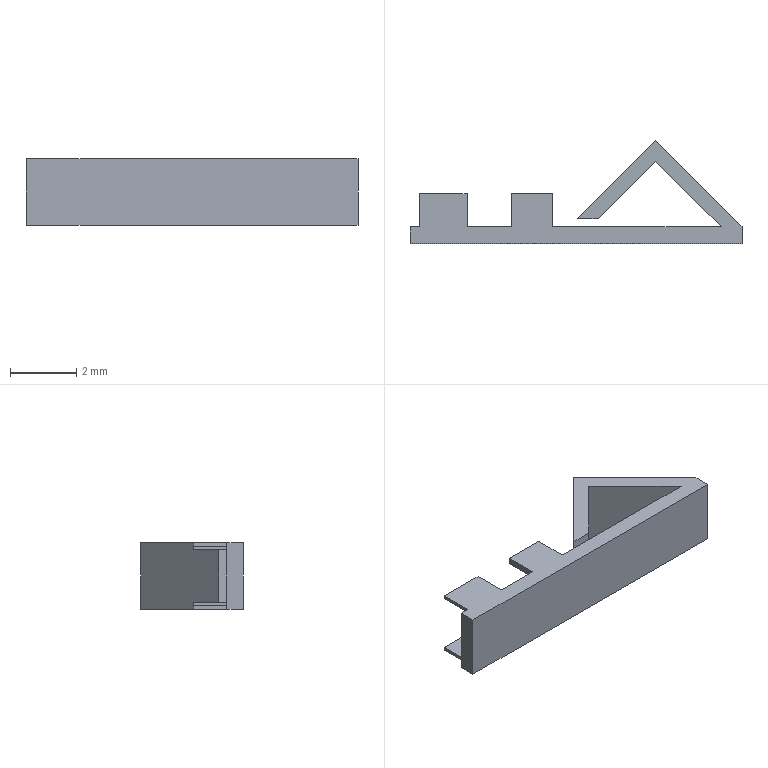Part | STEP file | 102000006964 | 1 solid | 27 faces | box 10 x 3.101 x 2 mm | volume 16.245 mm3 | plane 27
STEP:
#1=CARTESIAN_POINT('',(-9.435,0.5,0.));
#2=VERTEX_POINT('',#1);
#3=CARTESIAN_POINT('',(-9.435,0.5,0.2));
#4=VERTEX_POINT('',#3);
#5=CARTESIAN_POINT('',(-9.435,0.5,0.1));
#6=DIRECTION('',(0.,0.,1.));
#7=VECTOR('',#6,1.);
#8=LINE('',#5,#7);
#9=EDGE_CURVE('',#2,#4,#8,.T.);
#10=ORIENTED_EDGE('',*,*,#9,.F.);
#11=CARTESIAN_POINT('',(-10.775,0.5,0.));
#12=VERTEX_POINT('',#11);
#13=CARTESIAN_POINT('',(-10.105,0.5,0.));
#14=DIRECTION('',(-1.,0.,0.));
#15=VECTOR('',#14,1.);
#16=LINE('',#13,#15);
#17=EDGE_CURVE('',#2,#12,#16,.T.);
#18=ORIENTED_EDGE('',*,*,#17,.T.);
#19=CARTESIAN_POINT('',(-10.775,0.5,0.1));
#20=VERTEX_POINT('',#19);
#21=CARTESIAN_POINT('',(-10.775,0.5,0.05));
#22=DIRECTION('',(0.,0.,-1.));
#23=VECTOR('',#22,1.);
#24=LINE('',#21,#23);
#25=EDGE_CURVE('',#20,#12,#24,.T.);
#26=ORIENTED_EDGE('',*,*,#25,.F.);
#27=CARTESIAN_POINT('',(-12.211,0.5,0.1));
#28=VERTEX_POINT('',#27);
#29=CARTESIAN_POINT('',(-11.493,0.5,0.1));
#30=DIRECTION('',(1.,0.,0.));
#31=VECTOR('',#30,1.);
#32=LINE('',#29,#31);
#33=EDGE_CURVE('',#28,#20,#32,.T.);
#34=ORIENTED_EDGE('',*,*,#33,.F.);
#35=CARTESIAN_POINT('',(-12.211,0.5,0.));
#36=VERTEX_POINT('',#35);
#37=CARTESIAN_POINT('',(-12.211,0.5,0.05));
#38=DIRECTION('',(0.,0.,1.));
#39=VECTOR('',#38,1.);
#40=LINE('',#37,#39);
#41=EDGE_CURVE('',#36,#28,#40,.T.);
#42=ORIENTED_EDGE('',*,*,#41,.F.);
#43=CARTESIAN_POINT('',(-12.493,0.5,0.));
#44=VERTEX_POINT('',#43);
#45=CARTESIAN_POINT('',(-12.352,0.5,0.));
#46=DIRECTION('',(-1.,0.,0.));
#47=VECTOR('',#46,1.);
#48=LINE('',#45,#47);
#49=EDGE_CURVE('',#36,#44,#48,.T.);
#50=ORIENTED_EDGE('',*,*,#49,.T.);
#51=CARTESIAN_POINT('',(-12.493,0.5,2.));
#52=VERTEX_POINT('',#51);
#53=CARTESIAN_POINT('',(-12.493,0.5,1.));
#54=DIRECTION('',(0.,0.,-1.));
#55=VECTOR('',#54,1.);
#56=LINE('',#53,#55);
#57=EDGE_CURVE('',#52,#44,#56,.T.);
#58=ORIENTED_EDGE('',*,*,#57,.F.);
#59=CARTESIAN_POINT('',(-12.211,0.5,2.));
#60=VERTEX_POINT('',#59);
#61=CARTESIAN_POINT('',(-12.352,0.5,2.));
#62=DIRECTION('',(-1.,0.,0.));
#63=VECTOR('',#62,1.);
#64=LINE('',#61,#63);
#65=EDGE_CURVE('',#60,#52,#64,.T.);
#66=ORIENTED_EDGE('',*,*,#65,.F.);
#67=CARTESIAN_POINT('',(-12.211,0.5,1.9));
#68=VERTEX_POINT('',#67);
#69=CARTESIAN_POINT('',(-12.211,0.5,1.95));
#70=DIRECTION('',(0.,0.,1.));
#71=VECTOR('',#70,1.);
#72=LINE('',#69,#71);
#73=EDGE_CURVE('',#68,#60,#72,.T.);
#74=ORIENTED_EDGE('',*,*,#73,.F.);
#75=CARTESIAN_POINT('',(-10.775,0.5,1.9));
#76=VERTEX_POINT('',#75);
#77=CARTESIAN_POINT('',(-11.493,0.5,1.9));
#78=DIRECTION('',(-1.,0.,0.));
#79=VECTOR('',#78,1.);
#80=LINE('',#77,#79);
#81=EDGE_CURVE('',#76,#68,#80,.T.);
#82=ORIENTED_EDGE('',*,*,#81,.F.);
#83=CARTESIAN_POINT('',(-10.775,0.5,2.));
#84=VERTEX_POINT('',#83);
#85=CARTESIAN_POINT('',(-10.775,0.5,1.95));
#86=DIRECTION('',(0.,0.,-1.));
#87=VECTOR('',#86,1.);
#88=LINE('',#85,#87);
#89=EDGE_CURVE('',#84,#76,#88,.T.);
#90=ORIENTED_EDGE('',*,*,#89,.F.);
#91=CARTESIAN_POINT('',(-9.435,0.5,2.));
#92=VERTEX_POINT('',#91);
#93=CARTESIAN_POINT('',(-10.105,0.5,2.));
#94=DIRECTION('',(-1.,0.,0.));
#95=VECTOR('',#94,1.);
#96=LINE('',#93,#95);
#97=EDGE_CURVE('',#92,#84,#96,.T.);
#98=ORIENTED_EDGE('',*,*,#97,.F.);
#99=CARTESIAN_POINT('',(-9.435,0.5,1.8));
#100=VERTEX_POINT('',#99);
#101=CARTESIAN_POINT('',(-9.435,0.5,1.9));
#102=DIRECTION('',(0.,0.,1.));
#103=VECTOR('',#102,1.);
#104=LINE('',#101,#103);
#105=EDGE_CURVE('',#100,#92,#104,.T.);
#106=ORIENTED_EDGE('',*,*,#105,.F.);
#107=CARTESIAN_POINT('',(-8.19,0.5,1.8));
#108=VERTEX_POINT('',#107);
#109=CARTESIAN_POINT('',(-8.812,0.5,1.8));
#110=DIRECTION('',(-1.,0.,0.));
#111=VECTOR('',#110,1.);
#112=LINE('',#109,#111);
#113=EDGE_CURVE('',#108,#100,#112,.T.);
#114=ORIENTED_EDGE('',*,*,#113,.F.);
#115=CARTESIAN_POINT('',(-8.19,0.5,2.));
#116=VERTEX_POINT('',#115);
#117=CARTESIAN_POINT('',(-8.19,0.5,1.9));
#118=DIRECTION('',(0.,0.,-1.));
#119=VECTOR('',#118,1.);
#120=LINE('',#117,#119);
#121=EDGE_CURVE('',#116,#108,#120,.T.);
#122=ORIENTED_EDGE('',*,*,#121,.F.);
#123=CARTESIAN_POINT('',(-3.124,0.5,2.));
#124=VERTEX_POINT('',#123);
#125=CARTESIAN_POINT('',(-5.657,0.5,2.));
#126=DIRECTION('',(-1.,0.,0.));
#127=VECTOR('',#126,1.);
#128=LINE('',#125,#127);
#129=EDGE_CURVE('',#124,#116,#128,.T.);
#130=ORIENTED_EDGE('',*,*,#129,.F.);
#131=CARTESIAN_POINT('',(-3.124,0.5,0.));
#132=VERTEX_POINT('',#131);
#133=CARTESIAN_POINT('',(-3.124,0.5,1.));
#134=DIRECTION('',(0.,0.,1.));
#135=VECTOR('',#134,1.);
#136=LINE('',#133,#135);
#137=EDGE_CURVE('',#132,#124,#136,.T.);
#138=ORIENTED_EDGE('',*,*,#137,.F.);
#139=CARTESIAN_POINT('',(-8.19,0.5,0.));
#140=VERTEX_POINT('',#139);
#141=CARTESIAN_POINT('',(-5.657,0.5,0.));
#142=DIRECTION('',(-1.,0.,0.));
#143=VECTOR('',#142,1.);
#144=LINE('',#141,#143);
#145=EDGE_CURVE('',#132,#140,#144,.T.);
#146=ORIENTED_EDGE('',*,*,#145,.T.);
#147=CARTESIAN_POINT('',(-8.19,0.5,0.2));
#148=VERTEX_POINT('',#147);
#149=CARTESIAN_POINT('',(-8.19,0.5,0.1));
#150=DIRECTION('',(0.,0.,-1.));
#151=VECTOR('',#150,1.);
#152=LINE('',#149,#151);
#153=EDGE_CURVE('',#148,#140,#152,.T.);
#154=ORIENTED_EDGE('',*,*,#153,.F.);
#155=CARTESIAN_POINT('',(-8.812,0.5,0.2));
#156=DIRECTION('',(1.,0.,0.));
#157=VECTOR('',#156,1.);
#158=LINE('',#155,#157);
#159=EDGE_CURVE('',#4,#148,#158,.T.);
#160=ORIENTED_EDGE('',*,*,#159,.F.);
#161=EDGE_LOOP('',(#10,#18,#26,#34,#42,#50,#58,#66,#74,#82,#90,#98,#106,#114,#122,#130,#138,#146,#154,#160));
#162=FACE_OUTER_BOUND('',#161,.T.);
#163=CARTESIAN_POINT('',(-12.493,0.5,2.));
#164=DIRECTION('',(0.,-1.,0.));
#165=DIRECTION('',(1.,0.,0.));
#166=AXIS2_PLACEMENT_3D('',#163,#164,#165);
#167=PLANE('',#166);
#168=ADVANCED_FACE('',(#162),#167,.F.);
#169=ORIENTED_EDGE('',*,*,#9,.T.);
#170=CARTESIAN_POINT('',(-9.435,1.5,0.2));
#171=VERTEX_POINT('',#170);
#172=CARTESIAN_POINT('',(-9.435,1.,0.2));
#173=DIRECTION('',(0.,-1.,0.));
#174=VECTOR('',#173,1.);
#175=LINE('',#172,#174);
#176=EDGE_CURVE('',#171,#4,#175,.T.);
#177=ORIENTED_EDGE('',*,*,#176,.F.);
#178=CARTESIAN_POINT('',(-9.435,1.5,0.));
#179=VERTEX_POINT('',#178);
#180=CARTESIAN_POINT('',(-9.435,1.5,0.1));
#181=DIRECTION('',(0.,0.,1.));
#182=VECTOR('',#181,1.);
#183=LINE('',#180,#182);
#184=EDGE_CURVE('',#179,#171,#183,.T.);
#185=ORIENTED_EDGE('',*,*,#184,.F.);
#186=CARTESIAN_POINT('',(-9.435,1.,0.));
#187=DIRECTION('',(0.,-1.,0.));
#188=VECTOR('',#187,1.);
#189=LINE('',#186,#188);
#190=EDGE_CURVE('',#179,#2,#189,.T.);
#191=ORIENTED_EDGE('',*,*,#190,.T.);
#192=EDGE_LOOP('',(#169,#177,#185,#191));
#193=FACE_OUTER_BOUND('',#192,.T.);
#194=CARTESIAN_POINT('',(-9.435,1.5,0.));
#195=DIRECTION('',(1.,0.,0.));
#196=DIRECTION('',(0.,1.,0.));
#197=AXIS2_PLACEMENT_3D('',#194,#195,#196);
#198=PLANE('',#197);
#199=ADVANCED_FACE('',(#193),#198,.F.);
#200=CARTESIAN_POINT('',(-12.493,0.,0.));
#201=VERTEX_POINT('',#200);
#202=CARTESIAN_POINT('',(-12.493,0.25,0.));
#203=DIRECTION('',(0.,-1.,0.));
#204=VECTOR('',#203,1.);
#205=LINE('',#202,#204);
#206=EDGE_CURVE('',#44,#201,#205,.T.);
#207=ORIENTED_EDGE('',*,*,#206,.F.);
#208=ORIENTED_EDGE('',*,*,#49,.F.);
#209=CARTESIAN_POINT('',(-12.211,1.5,0.));
#210=VERTEX_POINT('',#209);
#211=CARTESIAN_POINT('',(-12.211,1.,0.));
#212=DIRECTION('',(0.,-1.,0.));
#213=VECTOR('',#212,1.);
#214=LINE('',#211,#213);
#215=EDGE_CURVE('',#210,#36,#214,.T.);
#216=ORIENTED_EDGE('',*,*,#215,.F.);
#217=CARTESIAN_POINT('',(-10.775,1.5,0.));
#218=VERTEX_POINT('',#217);
#219=CARTESIAN_POINT('',(-11.493,1.5,0.));
#220=DIRECTION('',(-1.,0.,0.));
#221=VECTOR('',#220,1.);
#222=LINE('',#219,#221);
#223=EDGE_CURVE('',#218,#210,#222,.T.);
#224=ORIENTED_EDGE('',*,*,#223,.F.);
#225=CARTESIAN_POINT('',(-10.775,1.,0.));
#226=DIRECTION('',(0.,-1.,0.));
#227=VECTOR('',#226,1.);
#228=LINE('',#225,#227);
#229=EDGE_CURVE('',#218,#12,#228,.T.);
#230=ORIENTED_EDGE('',*,*,#229,.T.);
#231=ORIENTED_EDGE('',*,*,#17,.F.);
#232=ORIENTED_EDGE('',*,*,#190,.F.);
#233=CARTESIAN_POINT('',(-8.19,1.5,0.));
#234=VERTEX_POINT('',#233);
#235=CARTESIAN_POINT('',(-8.812,1.5,0.));
#236=DIRECTION('',(-1.,0.,0.));
#237=VECTOR('',#236,1.);
#238=LINE('',#235,#237);
#239=EDGE_CURVE('',#234,#179,#238,.T.);
#240=ORIENTED_EDGE('',*,*,#239,.F.);
#241=CARTESIAN_POINT('',(-8.19,1.,0.));
#242=DIRECTION('',(0.,-1.,0.));
#243=VECTOR('',#242,1.);
#244=LINE('',#241,#243);
#245=EDGE_CURVE('',#234,#140,#244,.T.);
#246=ORIENTED_EDGE('',*,*,#245,.T.);
#247=ORIENTED_EDGE('',*,*,#145,.F.);
#248=CARTESIAN_POINT('',(-5.094,2.47,0.));
#249=VERTEX_POINT('',#248);
#250=CARTESIAN_POINT('',(-4.109,1.485,0.));
#251=DIRECTION('',(0.7071,-0.7071,0.));
#252=VECTOR('',#251,1.);
#253=LINE('',#250,#252);
#254=EDGE_CURVE('',#249,#132,#253,.T.);
#255=ORIENTED_EDGE('',*,*,#254,.F.);
#256=CARTESIAN_POINT('',(-6.823,0.7421,0.));
#257=VERTEX_POINT('',#256);
#258=CARTESIAN_POINT('',(-5.959,1.606,0.));
#259=DIRECTION('',(0.7071,0.7071,0.));
#260=VECTOR('',#259,1.);
#261=LINE('',#258,#260);
#262=EDGE_CURVE('',#257,#249,#261,.T.);
#263=ORIENTED_EDGE('',*,*,#262,.F.);
#264=CARTESIAN_POINT('',(-7.453,0.7421,0.));
#265=VERTEX_POINT('',#264);
#266=CARTESIAN_POINT('',(-7.138,0.7421,0.));
#267=DIRECTION('',(1.,0.,0.));
#268=VECTOR('',#267,1.);
#269=LINE('',#266,#268);
#270=EDGE_CURVE('',#265,#257,#269,.T.);
#271=ORIENTED_EDGE('',*,*,#270,.F.);
#272=CARTESIAN_POINT('',(-5.094,3.101,0.));
#273=VERTEX_POINT('',#272);
#274=CARTESIAN_POINT('',(-6.274,1.922,0.));
#275=DIRECTION('',(-0.7071,-0.7071,0.));
#276=VECTOR('',#275,1.);
#277=LINE('',#274,#276);
#278=EDGE_CURVE('',#273,#265,#277,.T.);
#279=ORIENTED_EDGE('',*,*,#278,.F.);
#280=CARTESIAN_POINT('',(-2.493,0.5,0.));
#281=VERTEX_POINT('',#280);
#282=CARTESIAN_POINT('',(-3.794,1.8,0.));
#283=DIRECTION('',(-0.7071,0.7071,0.));
#284=VECTOR('',#283,1.);
#285=LINE('',#282,#284);
#286=EDGE_CURVE('',#281,#273,#285,.T.);
#287=ORIENTED_EDGE('',*,*,#286,.F.);
#288=CARTESIAN_POINT('',(-2.493,0.,0.));
#289=VERTEX_POINT('',#288);
#290=CARTESIAN_POINT('',(-2.493,0.25,0.));
#291=DIRECTION('',(0.,1.,0.));
#292=VECTOR('',#291,1.);
#293=LINE('',#290,#292);
#294=EDGE_CURVE('',#289,#281,#293,.T.);
#295=ORIENTED_EDGE('',*,*,#294,.F.);
#296=CARTESIAN_POINT('',(-7.493,0.,0.));
#297=DIRECTION('',(1.,0.,0.));
#298=VECTOR('',#297,1.);
#299=LINE('',#296,#298);
#300=EDGE_CURVE('',#201,#289,#299,.T.);
#301=ORIENTED_EDGE('',*,*,#300,.F.);
#302=EDGE_LOOP('',(#207,#208,#216,#224,#230,#231,#232,#240,#246,#247,#255,#263,#271,#279,#287,#295,#301));
#303=FACE_OUTER_BOUND('',#302,.T.);
#304=CARTESIAN_POINT('',(0.,0.,0.));
#305=DIRECTION('',(0.,0.,1.));
#306=DIRECTION('',(1.,0.,0.));
#307=AXIS2_PLACEMENT_3D('',#304,#305,#306);
#308=PLANE('',#307);
#309=ADVANCED_FACE('',(#303),#308,.F.);
#310=ORIENTED_EDGE('',*,*,#25,.T.);
#311=ORIENTED_EDGE('',*,*,#229,.F.);
#312=CARTESIAN_POINT('',(-10.775,1.5,0.1));
#313=VERTEX_POINT('',#312);
#314=CARTESIAN_POINT('',(-10.775,1.5,0.05));
#315=DIRECTION('',(0.,0.,-1.));
#316=VECTOR('',#315,1.);
#317=LINE('',#314,#316);
#318=EDGE_CURVE('',#313,#218,#317,.T.);
#319=ORIENTED_EDGE('',*,*,#318,.F.);
#320=CARTESIAN_POINT('',(-10.775,1.,0.1));
#321=DIRECTION('',(0.,-1.,0.));
#322=VECTOR('',#321,1.);
#323=LINE('',#320,#322);
#324=EDGE_CURVE('',#313,#20,#323,.T.);
#325=ORIENTED_EDGE('',*,*,#324,.T.);
#326=EDGE_LOOP('',(#310,#311,#319,#325));
#327=FACE_OUTER_BOUND('',#326,.T.);
#328=CARTESIAN_POINT('',(-10.775,1.5,0.));
#329=DIRECTION('',(-1.,0.,0.));
#330=DIRECTION('',(0.,-1.,0.));
#331=AXIS2_PLACEMENT_3D('',#328,#329,#330);
#332=PLANE('',#331);
#333=ADVANCED_FACE('',(#327),#332,.F.);
#334=ORIENTED_EDGE('',*,*,#33,.T.);
#335=ORIENTED_EDGE('',*,*,#324,.F.);
#336=CARTESIAN_POINT('',(-12.211,1.5,0.1));
#337=VERTEX_POINT('',#336);
#338=CARTESIAN_POINT('',(-11.493,1.5,0.1));
#339=DIRECTION('',(1.,0.,0.));
#340=VECTOR('',#339,1.);
#341=LINE('',#338,#340);
#342=EDGE_CURVE('',#337,#313,#341,.T.);
#343=ORIENTED_EDGE('',*,*,#342,.F.);
#344=CARTESIAN_POINT('',(-12.211,1.,0.1));
#345=DIRECTION('',(0.,-1.,0.));
#346=VECTOR('',#345,1.);
#347=LINE('',#344,#346);
#348=EDGE_CURVE('',#337,#28,#347,.T.);
#349=ORIENTED_EDGE('',*,*,#348,.T.);
#350=EDGE_LOOP('',(#334,#335,#343,#349));
#351=FACE_OUTER_BOUND('',#350,.T.);
#352=CARTESIAN_POINT('',(-12.211,1.5,0.1));
#353=DIRECTION('',(0.,0.,-1.));
#354=DIRECTION('',(-1.,0.,0.));
#355=AXIS2_PLACEMENT_3D('',#352,#353,#354);
#356=PLANE('',#355);
#357=ADVANCED_FACE('',(#351),#356,.F.);
#358=ORIENTED_EDGE('',*,*,#41,.T.);
#359=ORIENTED_EDGE('',*,*,#348,.F.);
#360=CARTESIAN_POINT('',(-12.211,1.5,0.05));
#361=DIRECTION('',(0.,0.,1.));
#362=VECTOR('',#361,1.);
#363=LINE('',#360,#362);
#364=EDGE_CURVE('',#210,#337,#363,.T.);
#365=ORIENTED_EDGE('',*,*,#364,.F.);
#366=ORIENTED_EDGE('',*,*,#215,.T.);
#367=EDGE_LOOP('',(#358,#359,#365,#366));
#368=FACE_OUTER_BOUND('',#367,.T.);
#369=CARTESIAN_POINT('',(-12.211,1.5,0.));
#370=DIRECTION('',(1.,0.,0.));
#371=DIRECTION('',(0.,1.,0.));
#372=AXIS2_PLACEMENT_3D('',#369,#370,#371);
#373=PLANE('',#372);
#374=ADVANCED_FACE('',(#368),#373,.F.);
#375=ORIENTED_EDGE('',*,*,#206,.T.);
#376=CARTESIAN_POINT('',(-12.493,0.,2.));
#377=VERTEX_POINT('',#376);
#378=CARTESIAN_POINT('',(-12.493,0.,1.));
#379=DIRECTION('',(0.,0.,-1.));
#380=VECTOR('',#379,1.);
#381=LINE('',#378,#380);
#382=EDGE_CURVE('',#377,#201,#381,.T.);
#383=ORIENTED_EDGE('',*,*,#382,.F.);
#384=CARTESIAN_POINT('',(-12.493,0.25,2.));
#385=DIRECTION('',(0.,-1.,0.));
#386=VECTOR('',#385,1.);
#387=LINE('',#384,#386);
#388=EDGE_CURVE('',#52,#377,#387,.T.);
#389=ORIENTED_EDGE('',*,*,#388,.F.);
#390=ORIENTED_EDGE('',*,*,#57,.T.);
#391=EDGE_LOOP('',(#375,#383,#389,#390));
#392=FACE_OUTER_BOUND('',#391,.T.);
#393=CARTESIAN_POINT('',(-12.493,0.5,2.));
#394=DIRECTION('',(1.,0.,0.));
#395=DIRECTION('',(0.,0.,-1.));
#396=AXIS2_PLACEMENT_3D('',#393,#394,#395);
#397=PLANE('',#396);
#398=ADVANCED_FACE('',(#392),#397,.F.);
#399=ORIENTED_EDGE('',*,*,#388,.T.);
#400=CARTESIAN_POINT('',(-2.493,0.,2.));
#401=VERTEX_POINT('',#400);
#402=CARTESIAN_POINT('',(-7.493,0.,2.));
#403=DIRECTION('',(1.,0.,0.));
#404=VECTOR('',#403,1.);
#405=LINE('',#402,#404);
#406=EDGE_CURVE('',#377,#401,#405,.T.);
#407=ORIENTED_EDGE('',*,*,#406,.T.);
#408=CARTESIAN_POINT('',(-2.493,0.5,2.));
#409=VERTEX_POINT('',#408);
#410=CARTESIAN_POINT('',(-2.493,0.25,2.));
#411=DIRECTION('',(0.,1.,0.));
#412=VECTOR('',#411,1.);
#413=LINE('',#410,#412);
#414=EDGE_CURVE('',#401,#409,#413,.T.);
#415=ORIENTED_EDGE('',*,*,#414,.T.);
#416=CARTESIAN_POINT('',(-5.094,3.101,2.));
#417=VERTEX_POINT('',#416);
#418=CARTESIAN_POINT('',(-3.794,1.8,2.));
#419=DIRECTION('',(-0.7071,0.7071,0.));
#420=VECTOR('',#419,1.);
#421=LINE('',#418,#420);
#422=EDGE_CURVE('',#409,#417,#421,.T.);
#423=ORIENTED_EDGE('',*,*,#422,.T.);
#424=CARTESIAN_POINT('',(-7.453,0.7421,2.));
#425=VERTEX_POINT('',#424);
#426=CARTESIAN_POINT('',(-6.274,1.922,2.));
#427=DIRECTION('',(-0.7071,-0.7071,0.));
#428=VECTOR('',#427,1.);
#429=LINE('',#426,#428);
#430=EDGE_CURVE('',#417,#425,#429,.T.);
#431=ORIENTED_EDGE('',*,*,#430,.T.);
#432=CARTESIAN_POINT('',(-6.823,0.7421,2.));
#433=VERTEX_POINT('',#432);
#434=CARTESIAN_POINT('',(-7.138,0.7421,2.));
#435=DIRECTION('',(1.,0.,0.));
#436=VECTOR('',#435,1.);
#437=LINE('',#434,#436);
#438=EDGE_CURVE('',#425,#433,#437,.T.);
#439=ORIENTED_EDGE('',*,*,#438,.T.);
#440=CARTESIAN_POINT('',(-5.094,2.47,2.));
#441=VERTEX_POINT('',#440);
#442=CARTESIAN_POINT('',(-5.959,1.606,2.));
#443=DIRECTION('',(0.7071,0.7071,0.));
#444=VECTOR('',#443,1.);
#445=LINE('',#442,#444);
#446=EDGE_CURVE('',#433,#441,#445,.T.);
#447=ORIENTED_EDGE('',*,*,#446,.T.);
#448=CARTESIAN_POINT('',(-4.109,1.485,2.));
#449=DIRECTION('',(0.7071,-0.7071,0.));
#450=VECTOR('',#449,1.);
#451=LINE('',#448,#450);
#452=EDGE_CURVE('',#441,#124,#451,.T.);
#453=ORIENTED_EDGE('',*,*,#452,.T.);
#454=ORIENTED_EDGE('',*,*,#129,.T.);
#455=CARTESIAN_POINT('',(-8.19,1.5,2.));
#456=VERTEX_POINT('',#455);
#457=CARTESIAN_POINT('',(-8.19,1.,2.));
#458=DIRECTION('',(0.,-1.,0.));
#459=VECTOR('',#458,1.);
#460=LINE('',#457,#459);
#461=EDGE_CURVE('',#456,#116,#460,.T.);
#462=ORIENTED_EDGE('',*,*,#461,.F.);
#463=CARTESIAN_POINT('',(-9.435,1.5,2.));
#464=VERTEX_POINT('',#463);
#465=CARTESIAN_POINT('',(-8.812,1.5,2.));
#466=DIRECTION('',(1.,0.,0.));
#467=VECTOR('',#466,1.);
#468=LINE('',#465,#467);
#469=EDGE_CURVE('',#464,#456,#468,.T.);
#470=ORIENTED_EDGE('',*,*,#469,.F.);
#471=CARTESIAN_POINT('',(-9.435,1.,2.));
#472=DIRECTION('',(0.,-1.,0.));
#473=VECTOR('',#472,1.);
#474=LINE('',#471,#473);
#475=EDGE_CURVE('',#464,#92,#474,.T.);
#476=ORIENTED_EDGE('',*,*,#475,.T.);
#477=ORIENTED_EDGE('',*,*,#97,.T.);
#478=CARTESIAN_POINT('',(-10.775,1.5,2.));
#479=VERTEX_POINT('',#478);
#480=CARTESIAN_POINT('',(-10.775,1.,2.));
#481=DIRECTION('',(0.,-1.,0.));
#482=VECTOR('',#481,1.);
#483=LINE('',#480,#482);
#484=EDGE_CURVE('',#479,#84,#483,.T.);
#485=ORIENTED_EDGE('',*,*,#484,.F.);
#486=CARTESIAN_POINT('',(-12.211,1.5,2.));
#487=VERTEX_POINT('',#486);
#488=CARTESIAN_POINT('',(-11.493,1.5,2.));
#489=DIRECTION('',(1.,0.,0.));
#490=VECTOR('',#489,1.);
#491=LINE('',#488,#490);
#492=EDGE_CURVE('',#487,#479,#491,.T.);
#493=ORIENTED_EDGE('',*,*,#492,.F.);
#494=CARTESIAN_POINT('',(-12.211,1.,2.));
#495=DIRECTION('',(0.,-1.,0.));
#496=VECTOR('',#495,1.);
#497=LINE('',#494,#496);
#498=EDGE_CURVE('',#487,#60,#497,.T.);
#499=ORIENTED_EDGE('',*,*,#498,.T.);
#500=ORIENTED_EDGE('',*,*,#65,.T.);
#501=EDGE_LOOP('',(#399,#407,#415,#423,#431,#439,#447,#453,#454,#462,#470,#476,#477,#485,#493,#499,#500));
#502=FACE_OUTER_BOUND('',#501,.T.);
#503=CARTESIAN_POINT('',(0.,0.,2.));
#504=DIRECTION('',(0.,0.,1.));
#505=DIRECTION('',(1.,0.,0.));
#506=AXIS2_PLACEMENT_3D('',#503,#504,#505);
#507=PLANE('',#506);
#508=ADVANCED_FACE('',(#502),#507,.T.);
#509=ORIENTED_EDGE('',*,*,#73,.T.);
#510=ORIENTED_EDGE('',*,*,#498,.F.);
#511=CARTESIAN_POINT('',(-12.211,1.5,1.9));
#512=VERTEX_POINT('',#511);
#513=CARTESIAN_POINT('',(-12.211,1.5,1.95));
#514=DIRECTION('',(0.,0.,1.));
#515=VECTOR('',#514,1.);
#516=LINE('',#513,#515);
#517=EDGE_CURVE('',#512,#487,#516,.T.);
#518=ORIENTED_EDGE('',*,*,#517,.F.);
#519=CARTESIAN_POINT('',(-12.211,1.,1.9));
#520=DIRECTION('',(0.,-1.,0.));
#521=VECTOR('',#520,1.);
#522=LINE('',#519,#521);
#523=EDGE_CURVE('',#512,#68,#522,.T.);
#524=ORIENTED_EDGE('',*,*,#523,.T.);
#525=EDGE_LOOP('',(#509,#510,#518,#524));
#526=FACE_OUTER_BOUND('',#525,.T.);
#527=CARTESIAN_POINT('',(-12.211,1.5,2.));
#528=DIRECTION('',(1.,0.,0.));
#529=DIRECTION('',(0.,1.,0.));
#530=AXIS2_PLACEMENT_3D('',#527,#528,#529);
#531=PLANE('',#530);
#532=ADVANCED_FACE('',(#526),#531,.F.);
#533=ORIENTED_EDGE('',*,*,#81,.T.);
#534=ORIENTED_EDGE('',*,*,#523,.F.);
#535=CARTESIAN_POINT('',(-10.775,1.5,1.9));
#536=VERTEX_POINT('',#535);
#537=CARTESIAN_POINT('',(-11.493,1.5,1.9));
#538=DIRECTION('',(-1.,0.,0.));
#539=VECTOR('',#538,1.);
#540=LINE('',#537,#539);
#541=EDGE_CURVE('',#536,#512,#540,.T.);
#542=ORIENTED_EDGE('',*,*,#541,.F.);
#543=CARTESIAN_POINT('',(-10.775,1.,1.9));
#544=DIRECTION('',(0.,-1.,0.));
#545=VECTOR('',#544,1.);
#546=LINE('',#543,#545);
#547=EDGE_CURVE('',#536,#76,#546,.T.);
#548=ORIENTED_EDGE('',*,*,#547,.T.);
#549=EDGE_LOOP('',(#533,#534,#542,#548));
#550=FACE_OUTER_BOUND('',#549,.T.);
#551=CARTESIAN_POINT('',(-12.211,1.5,1.9));
#552=DIRECTION('',(0.,0.,1.));
#553=DIRECTION('',(1.,0.,0.));
#554=AXIS2_PLACEMENT_3D('',#551,#552,#553);
#555=PLANE('',#554);
#556=ADVANCED_FACE('',(#550),#555,.F.);
#557=ORIENTED_EDGE('',*,*,#89,.T.);
#558=ORIENTED_EDGE('',*,*,#547,.F.);
#559=CARTESIAN_POINT('',(-10.775,1.5,1.95));
#560=DIRECTION('',(0.,0.,-1.));
#561=VECTOR('',#560,1.);
#562=LINE('',#559,#561);
#563=EDGE_CURVE('',#479,#536,#562,.T.);
#564=ORIENTED_EDGE('',*,*,#563,.F.);
#565=ORIENTED_EDGE('',*,*,#484,.T.);
#566=EDGE_LOOP('',(#557,#558,#564,#565));
#567=FACE_OUTER_BOUND('',#566,.T.);
#568=CARTESIAN_POINT('',(-10.775,1.5,2.));
#569=DIRECTION('',(-1.,0.,0.));
#570=DIRECTION('',(0.,-1.,0.));
#571=AXIS2_PLACEMENT_3D('',#568,#569,#570);
#572=PLANE('',#571);
#573=ADVANCED_FACE('',(#567),#572,.F.);
#574=ORIENTED_EDGE('',*,*,#105,.T.);
#575=ORIENTED_EDGE('',*,*,#475,.F.);
#576=CARTESIAN_POINT('',(-9.435,1.5,1.8));
#577=VERTEX_POINT('',#576);
#578=CARTESIAN_POINT('',(-9.435,1.5,1.9));
#579=DIRECTION('',(0.,0.,1.));
#580=VECTOR('',#579,1.);
#581=LINE('',#578,#580);
#582=EDGE_CURVE('',#577,#464,#581,.T.);
#583=ORIENTED_EDGE('',*,*,#582,.F.);
#584=CARTESIAN_POINT('',(-9.435,1.,1.8));
#585=DIRECTION('',(0.,-1.,0.));
#586=VECTOR('',#585,1.);
#587=LINE('',#584,#586);
#588=EDGE_CURVE('',#577,#100,#587,.T.);
#589=ORIENTED_EDGE('',*,*,#588,.T.);
#590=EDGE_LOOP('',(#574,#575,#583,#589));
#591=FACE_OUTER_BOUND('',#590,.T.);
#592=CARTESIAN_POINT('',(-9.435,1.5,2.));
#593=DIRECTION('',(1.,0.,0.));
#594=DIRECTION('',(0.,1.,0.));
#595=AXIS2_PLACEMENT_3D('',#592,#593,#594);
#596=PLANE('',#595);
#597=ADVANCED_FACE('',(#591),#596,.F.);
#598=ORIENTED_EDGE('',*,*,#113,.T.);
#599=ORIENTED_EDGE('',*,*,#588,.F.);
#600=CARTESIAN_POINT('',(-8.19,1.5,1.8));
#601=VERTEX_POINT('',#600);
#602=CARTESIAN_POINT('',(-8.812,1.5,1.8));
#603=DIRECTION('',(-1.,0.,0.));
#604=VECTOR('',#603,1.);
#605=LINE('',#602,#604);
#606=EDGE_CURVE('',#601,#577,#605,.T.);
#607=ORIENTED_EDGE('',*,*,#606,.F.);
#608=CARTESIAN_POINT('',(-8.19,1.,1.8));
#609=DIRECTION('',(0.,-1.,0.));
#610=VECTOR('',#609,1.);
#611=LINE('',#608,#610);
#612=EDGE_CURVE('',#601,#108,#611,.T.);
#613=ORIENTED_EDGE('',*,*,#612,.T.);
#614=EDGE_LOOP('',(#598,#599,#607,#613));
#615=FACE_OUTER_BOUND('',#614,.T.);
#616=CARTESIAN_POINT('',(-9.435,1.5,1.8));
#617=DIRECTION('',(0.,0.,1.));
#618=DIRECTION('',(1.,0.,0.));
#619=AXIS2_PLACEMENT_3D('',#616,#617,#618);
#620=PLANE('',#619);
#621=ADVANCED_FACE('',(#615),#620,.F.);
#622=ORIENTED_EDGE('',*,*,#121,.T.);
#623=ORIENTED_EDGE('',*,*,#612,.F.);
#624=CARTESIAN_POINT('',(-8.19,1.5,1.9));
#625=DIRECTION('',(0.,0.,-1.));
#626=VECTOR('',#625,1.);
#627=LINE('',#624,#626);
#628=EDGE_CURVE('',#456,#601,#627,.T.);
#629=ORIENTED_EDGE('',*,*,#628,.F.);
#630=ORIENTED_EDGE('',*,*,#461,.T.);
#631=EDGE_LOOP('',(#622,#623,#629,#630));
#632=FACE_OUTER_BOUND('',#631,.T.);
#633=CARTESIAN_POINT('',(-8.19,1.5,2.));
#634=DIRECTION('',(-1.,0.,0.));
#635=DIRECTION('',(0.,-1.,0.));
#636=AXIS2_PLACEMENT_3D('',#633,#634,#635);
#637=PLANE('',#636);
#638=ADVANCED_FACE('',(#632),#637,.F.);
#639=ORIENTED_EDGE('',*,*,#452,.F.);
#640=CARTESIAN_POINT('',(-5.094,2.47,1.));
#641=DIRECTION('',(0.,0.,1.));
#642=VECTOR('',#641,1.);
#643=LINE('',#640,#642);
#644=EDGE_CURVE('',#249,#441,#643,.T.);
#645=ORIENTED_EDGE('',*,*,#644,.F.);
#646=ORIENTED_EDGE('',*,*,#254,.T.);
#647=ORIENTED_EDGE('',*,*,#137,.T.);
#648=EDGE_LOOP('',(#639,#645,#646,#647));
#649=FACE_OUTER_BOUND('',#648,.T.);
#650=CARTESIAN_POINT('',(-5.094,2.47,0.));
#651=DIRECTION('',(-0.7071,-0.7071,0.));
#652=DIRECTION('',(0.7071,-0.7071,0.));
#653=AXIS2_PLACEMENT_3D('',#650,#651,#652);
#654=PLANE('',#653);
#655=ADVANCED_FACE('',(#649),#654,.T.);
#656=ORIENTED_EDGE('',*,*,#153,.T.);
#657=ORIENTED_EDGE('',*,*,#245,.F.);
#658=CARTESIAN_POINT('',(-8.19,1.5,0.2));
#659=VERTEX_POINT('',#658);
#660=CARTESIAN_POINT('',(-8.19,1.5,0.1));
#661=DIRECTION('',(0.,0.,-1.));
#662=VECTOR('',#661,1.);
#663=LINE('',#660,#662);
#664=EDGE_CURVE('',#659,#234,#663,.T.);
#665=ORIENTED_EDGE('',*,*,#664,.F.);
#666=CARTESIAN_POINT('',(-8.19,1.,0.2));
#667=DIRECTION('',(0.,-1.,0.));
#668=VECTOR('',#667,1.);
#669=LINE('',#666,#668);
#670=EDGE_CURVE('',#659,#148,#669,.T.);
#671=ORIENTED_EDGE('',*,*,#670,.T.);
#672=EDGE_LOOP('',(#656,#657,#665,#671));
#673=FACE_OUTER_BOUND('',#672,.T.);
#674=CARTESIAN_POINT('',(-8.19,1.5,0.));
#675=DIRECTION('',(-1.,0.,0.));
#676=DIRECTION('',(0.,-1.,0.));
#677=AXIS2_PLACEMENT_3D('',#674,#675,#676);
#678=PLANE('',#677);
#679=ADVANCED_FACE('',(#673),#678,.F.);
#680=ORIENTED_EDGE('',*,*,#159,.T.);
#681=ORIENTED_EDGE('',*,*,#670,.F.);
#682=CARTESIAN_POINT('',(-8.812,1.5,0.2));
#683=DIRECTION('',(1.,0.,0.));
#684=VECTOR('',#683,1.);
#685=LINE('',#682,#684);
#686=EDGE_CURVE('',#171,#659,#685,.T.);
#687=ORIENTED_EDGE('',*,*,#686,.F.);
#688=ORIENTED_EDGE('',*,*,#176,.T.);
#689=EDGE_LOOP('',(#680,#681,#687,#688));
#690=FACE_OUTER_BOUND('',#689,.T.);
#691=CARTESIAN_POINT('',(-9.435,1.5,0.2));
#692=DIRECTION('',(0.,0.,-1.));
#693=DIRECTION('',(-1.,0.,0.));
#694=AXIS2_PLACEMENT_3D('',#691,#692,#693);
#695=PLANE('',#694);
#696=ADVANCED_FACE('',(#690),#695,.F.);
#697=ORIENTED_EDGE('',*,*,#184,.T.);
#698=ORIENTED_EDGE('',*,*,#686,.T.);
#699=ORIENTED_EDGE('',*,*,#664,.T.);
#700=ORIENTED_EDGE('',*,*,#239,.T.);
#701=EDGE_LOOP('',(#697,#698,#699,#700));
#702=FACE_OUTER_BOUND('',#701,.T.);
#703=CARTESIAN_POINT('',(0.,1.5,0.));
#704=DIRECTION('',(0.,1.,0.));
#705=DIRECTION('',(-1.,0.,0.));
#706=AXIS2_PLACEMENT_3D('',#703,#704,#705);
#707=PLANE('',#706);
#708=ADVANCED_FACE('',(#702),#707,.T.);
#709=ORIENTED_EDGE('',*,*,#364,.T.);
#710=ORIENTED_EDGE('',*,*,#342,.T.);
#711=ORIENTED_EDGE('',*,*,#318,.T.);
#712=ORIENTED_EDGE('',*,*,#223,.T.);
#713=EDGE_LOOP('',(#709,#710,#711,#712));
#714=FACE_OUTER_BOUND('',#713,.T.);
#715=CARTESIAN_POINT('',(0.,1.5,0.));
#716=DIRECTION('',(0.,1.,0.));
#717=DIRECTION('',(-1.,0.,0.));
#718=AXIS2_PLACEMENT_3D('',#715,#716,#717);
#719=PLANE('',#718);
#720=ADVANCED_FACE('',(#714),#719,.T.);
#721=ORIENTED_EDGE('',*,*,#446,.F.);
#722=CARTESIAN_POINT('',(-6.823,0.7421,1.));
#723=DIRECTION('',(0.,0.,1.));
#724=VECTOR('',#723,1.);
#725=LINE('',#722,#724);
#726=EDGE_CURVE('',#257,#433,#725,.T.);
#727=ORIENTED_EDGE('',*,*,#726,.F.);
#728=ORIENTED_EDGE('',*,*,#262,.T.);
#729=ORIENTED_EDGE('',*,*,#644,.T.);
#730=EDGE_LOOP('',(#721,#727,#728,#729));
#731=FACE_OUTER_BOUND('',#730,.T.);
#732=CARTESIAN_POINT('',(-6.823,0.7421,0.));
#733=DIRECTION('',(0.7071,-0.7071,0.));
#734=DIRECTION('',(0.7071,0.7071,0.));
#735=AXIS2_PLACEMENT_3D('',#732,#733,#734);
#736=PLANE('',#735);
#737=ADVANCED_FACE('',(#731),#736,.T.);
#738=ORIENTED_EDGE('',*,*,#438,.F.);
#739=CARTESIAN_POINT('',(-7.453,0.7421,1.));
#740=DIRECTION('',(0.,0.,1.));
#741=VECTOR('',#740,1.);
#742=LINE('',#739,#741);
#743=EDGE_CURVE('',#265,#425,#742,.T.);
#744=ORIENTED_EDGE('',*,*,#743,.F.);
#745=ORIENTED_EDGE('',*,*,#270,.T.);
#746=ORIENTED_EDGE('',*,*,#726,.T.);
#747=EDGE_LOOP('',(#738,#744,#745,#746));
#748=FACE_OUTER_BOUND('',#747,.T.);
#749=CARTESIAN_POINT('',(-7.453,0.7421,0.));
#750=DIRECTION('',(0.,-1.,0.));
#751=DIRECTION('',(0.,0.,-1.));
#752=AXIS2_PLACEMENT_3D('',#749,#750,#751);
#753=PLANE('',#752);
#754=ADVANCED_FACE('',(#748),#753,.T.);
#755=ORIENTED_EDGE('',*,*,#430,.F.);
#756=CARTESIAN_POINT('',(-5.094,3.101,1.));
#757=DIRECTION('',(0.,0.,1.));
#758=VECTOR('',#757,1.);
#759=LINE('',#756,#758);
#760=EDGE_CURVE('',#273,#417,#759,.T.);
#761=ORIENTED_EDGE('',*,*,#760,.F.);
#762=ORIENTED_EDGE('',*,*,#278,.T.);
#763=ORIENTED_EDGE('',*,*,#743,.T.);
#764=EDGE_LOOP('',(#755,#761,#762,#763));
#765=FACE_OUTER_BOUND('',#764,.T.);
#766=CARTESIAN_POINT('',(-5.094,3.101,0.));
#767=DIRECTION('',(-0.7071,0.7071,0.));
#768=DIRECTION('',(-0.7071,-0.7071,0.));
#769=AXIS2_PLACEMENT_3D('',#766,#767,#768);
#770=PLANE('',#769);
#771=ADVANCED_FACE('',(#765),#770,.T.);
#772=ORIENTED_EDGE('',*,*,#422,.F.);
#773=CARTESIAN_POINT('',(-2.493,0.5,1.));
#774=DIRECTION('',(0.,0.,-1.));
#775=VECTOR('',#774,1.);
#776=LINE('',#773,#775);
#777=EDGE_CURVE('',#409,#281,#776,.T.);
#778=ORIENTED_EDGE('',*,*,#777,.T.);
#779=ORIENTED_EDGE('',*,*,#286,.T.);
#780=ORIENTED_EDGE('',*,*,#760,.T.);
#781=EDGE_LOOP('',(#772,#778,#779,#780));
#782=FACE_OUTER_BOUND('',#781,.T.);
#783=CARTESIAN_POINT('',(-2.493,0.5,0.));
#784=DIRECTION('',(0.7071,0.7071,0.));
#785=DIRECTION('',(-0.7071,0.7071,0.));
#786=AXIS2_PLACEMENT_3D('',#783,#784,#785);
#787=PLANE('',#786);
#788=ADVANCED_FACE('',(#782),#787,.T.);
#789=ORIENTED_EDGE('',*,*,#294,.T.);
#790=ORIENTED_EDGE('',*,*,#777,.F.);
#791=ORIENTED_EDGE('',*,*,#414,.F.);
#792=CARTESIAN_POINT('',(-2.493,0.,1.));
#793=DIRECTION('',(0.,0.,-1.));
#794=VECTOR('',#793,1.);
#795=LINE('',#792,#794);
#796=EDGE_CURVE('',#401,#289,#795,.T.);
#797=ORIENTED_EDGE('',*,*,#796,.T.);
#798=EDGE_LOOP('',(#789,#790,#791,#797));
#799=FACE_OUTER_BOUND('',#798,.T.);
#800=CARTESIAN_POINT('',(-2.493,0.5,2.));
#801=DIRECTION('',(-1.,0.,0.));
#802=DIRECTION('',(0.,0.,1.));
#803=AXIS2_PLACEMENT_3D('',#800,#801,#802);
#804=PLANE('',#803);
#805=ADVANCED_FACE('',(#799),#804,.F.);
#806=ORIENTED_EDGE('',*,*,#300,.T.);
#807=ORIENTED_EDGE('',*,*,#796,.F.);
#808=ORIENTED_EDGE('',*,*,#406,.F.);
#809=ORIENTED_EDGE('',*,*,#382,.T.);
#810=EDGE_LOOP('',(#806,#807,#808,#809));
#811=FACE_OUTER_BOUND('',#810,.T.);
#812=CARTESIAN_POINT('',(-12.493,0.,2.));
#813=DIRECTION('',(0.,1.,0.));
#814=DIRECTION('',(0.,0.,1.));
#815=AXIS2_PLACEMENT_3D('',#812,#813,#814);
#816=PLANE('',#815);
#817=ADVANCED_FACE('',(#811),#816,.F.);
#818=ORIENTED_EDGE('',*,*,#582,.T.);
#819=ORIENTED_EDGE('',*,*,#469,.T.);
#820=ORIENTED_EDGE('',*,*,#628,.T.);
#821=ORIENTED_EDGE('',*,*,#606,.T.);
#822=EDGE_LOOP('',(#818,#819,#820,#821));
#823=FACE_OUTER_BOUND('',#822,.T.);
#824=CARTESIAN_POINT('',(0.,1.5,0.));
#825=DIRECTION('',(0.,-1.,0.));
#826=DIRECTION('',(1.,0.,0.));
#827=AXIS2_PLACEMENT_3D('',#824,#825,#826);
#828=PLANE('',#827);
#829=ADVANCED_FACE('',(#823),#828,.F.);
#830=ORIENTED_EDGE('',*,*,#517,.T.);
#831=ORIENTED_EDGE('',*,*,#492,.T.);
#832=ORIENTED_EDGE('',*,*,#563,.T.);
#833=ORIENTED_EDGE('',*,*,#541,.T.);
#834=EDGE_LOOP('',(#830,#831,#832,#833));
#835=FACE_OUTER_BOUND('',#834,.T.);
#836=CARTESIAN_POINT('',(0.,1.5,0.));
#837=DIRECTION('',(0.,-1.,0.));
#838=DIRECTION('',(1.,0.,0.));
#839=AXIS2_PLACEMENT_3D('',#836,#837,#838);
#840=PLANE('',#839);
#841=ADVANCED_FACE('',(#835),#840,.F.);
#842=CLOSED_SHELL('',(#168,#199,#309,#333,#357,#374,#398,#508,#532,#556,#573,#597,#621,#638,#655,#679,#696,#708,#720,#737,#754,#771,#788,#805,#817,#829,#841));
#843=MANIFOLD_SOLID_BREP('',#842);
#844=(LENGTH_UNIT()NAMED_UNIT(*)SI_UNIT(.MILLI.,.METRE.));
#845=UNCERTAINTY_MEASURE_WITH_UNIT(LENGTH_MEASURE(0.005),#844,'','');
#846=(NAMED_UNIT(*)PLANE_ANGLE_UNIT()SI_UNIT($,.RADIAN.));
#847=(NAMED_UNIT(*)SI_UNIT($,.STERADIAN.)SOLID_ANGLE_UNIT());
#848=(GEOMETRIC_REPRESENTATION_CONTEXT(3)GLOBAL_UNCERTAINTY_ASSIGNED_CONTEXT((#845))GLOBAL_UNIT_ASSIGNED_CONTEXT((#844,#846,#847))REPRESENTATION_CONTEXT('',''));
#849=ADVANCED_BREP_SHAPE_REPRESENTATION('',(#843),#848);